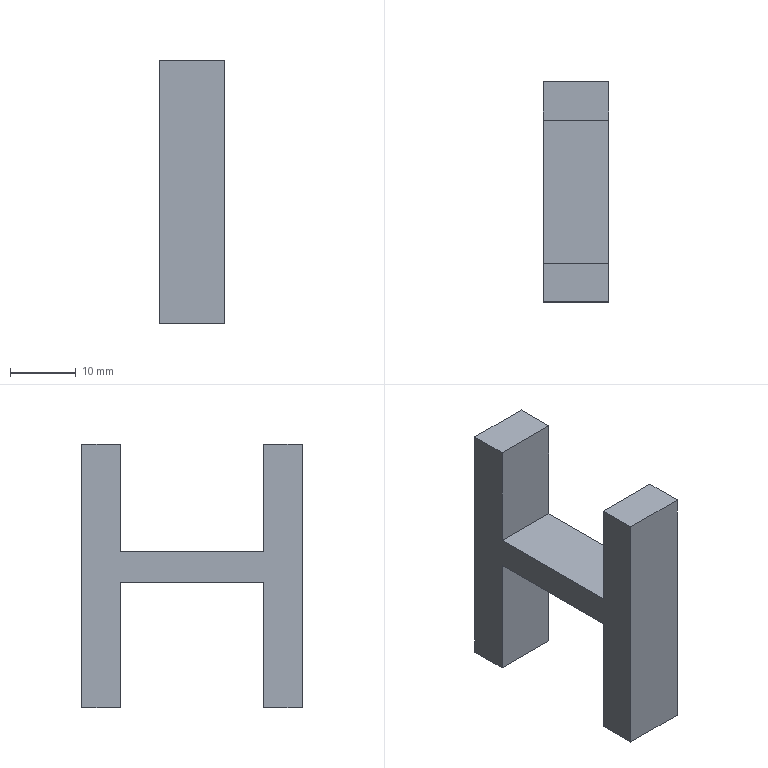Part | NX | features solid 2 | 1 solid | 14 faces | box 10 x 33.468 x 40 mm | volume 5698 mm3 | plane 14
STEP:
#1=CARTESIAN_POINT('',(2250.,-874.141,-590.));
#2=VERTEX_POINT('',#1);
#3=CARTESIAN_POINT('',(2250.,-880.,-590.));
#4=VERTEX_POINT('',#3);
#5=CARTESIAN_POINT('',(2250.,-874.141,-590.));
#6=CARTESIAN_POINT('',(2250.,-876.094,-590.));
#7=CARTESIAN_POINT('',(2250.,-878.047,-590.));
#8=CARTESIAN_POINT('',(2250.,-880.,-590.));
#9=B_SPLINE_CURVE_WITH_KNOTS('',3,(#5,#6,#7,#8),.UNSPECIFIED.,.F.,.F.,(4,4),(0.,0.02692),.PIECEWISE_BEZIER_KNOTS.);
#10=EDGE_CURVE('',#2,#4,#9,.T.);
#11=ORIENTED_EDGE('',*,*,#10,.F.);
#12=CARTESIAN_POINT('',(2260.,-874.141,-590.));
#13=VERTEX_POINT('',#12);
#14=CARTESIAN_POINT('',(2260.,-874.141,-590.));
#15=DIRECTION('',(-1.,0.,0.));
#16=VECTOR('',#15,1000.);
#17=LINE('',#14,#16);
#18=EDGE_CURVE('',#13,#2,#17,.T.);
#19=ORIENTED_EDGE('',*,*,#18,.F.);
#20=CARTESIAN_POINT('',(2260.,-880.,-590.));
#21=VERTEX_POINT('',#20);
#22=CARTESIAN_POINT('',(2260.,-874.141,-590.));
#23=CARTESIAN_POINT('',(2260.,-876.094,-590.));
#24=CARTESIAN_POINT('',(2260.,-878.047,-590.));
#25=CARTESIAN_POINT('',(2260.,-880.,-590.));
#26=B_SPLINE_CURVE_WITH_KNOTS('',3,(#22,#23,#24,#25),.UNSPECIFIED.,.F.,.F.,(4,4),(0.,0.02692),.PIECEWISE_BEZIER_KNOTS.);
#27=EDGE_CURVE('',#13,#21,#26,.T.);
#28=ORIENTED_EDGE('',*,*,#27,.T.);
#29=CARTESIAN_POINT('',(2260.,-880.,-590.));
#30=DIRECTION('',(-1.,0.,0.));
#31=VECTOR('',#30,1000.);
#32=LINE('',#29,#31);
#33=EDGE_CURVE('',#21,#4,#32,.T.);
#34=ORIENTED_EDGE('',*,*,#33,.T.);
#35=EDGE_LOOP('',(#11,#19,#28,#34));
#36=FACE_BOUND('',#35,.T.);
#37=CARTESIAN_POINT('',(2260.,-874.141,-590.));
#38=DIRECTION('',(0.,0.,-1.));
#39=DIRECTION('',(-1.,0.,0.));
#40=AXIS2_PLACEMENT_3D('',#37,#38,#39);
#41=PLANE('',#40);
#42=ADVANCED_FACE('',(#36),#41,.T.);
#43=CARTESIAN_POINT('',(2250.,-880.,-550.));
#44=VERTEX_POINT('',#43);
#45=CARTESIAN_POINT('',(2250.,-880.,-590.));
#46=CARTESIAN_POINT('',(2250.,-880.,-576.667));
#47=CARTESIAN_POINT('',(2250.,-880.,-563.333));
#48=CARTESIAN_POINT('',(2250.,-880.,-550.));
#49=B_SPLINE_CURVE_WITH_KNOTS('',3,(#45,#46,#47,#48),.UNSPECIFIED.,.F.,.F.,(4,4),(0.02692,0.2107),.PIECEWISE_BEZIER_KNOTS.);
#50=EDGE_CURVE('',#4,#44,#49,.T.);
#51=ORIENTED_EDGE('',*,*,#50,.F.);
#52=ORIENTED_EDGE('',*,*,#33,.F.);
#53=CARTESIAN_POINT('',(2260.,-880.,-550.));
#54=VERTEX_POINT('',#53);
#55=CARTESIAN_POINT('',(2260.,-880.,-590.));
#56=CARTESIAN_POINT('',(2260.,-880.,-576.667));
#57=CARTESIAN_POINT('',(2260.,-880.,-563.333));
#58=CARTESIAN_POINT('',(2260.,-880.,-550.));
#59=B_SPLINE_CURVE_WITH_KNOTS('',3,(#55,#56,#57,#58),.UNSPECIFIED.,.F.,.F.,(4,4),(0.02692,0.2107),.PIECEWISE_BEZIER_KNOTS.);
#60=EDGE_CURVE('',#21,#54,#59,.T.);
#61=ORIENTED_EDGE('',*,*,#60,.T.);
#62=CARTESIAN_POINT('',(2260.,-880.,-550.));
#63=DIRECTION('',(-1.,0.,0.));
#64=VECTOR('',#63,1000.);
#65=LINE('',#62,#64);
#66=EDGE_CURVE('',#54,#44,#65,.T.);
#67=ORIENTED_EDGE('',*,*,#66,.T.);
#68=EDGE_LOOP('',(#51,#52,#61,#67));
#69=FACE_BOUND('',#68,.T.);
#70=CARTESIAN_POINT('',(2260.,-880.,-590.));
#71=DIRECTION('',(0.,-1.,0.));
#72=DIRECTION('',(1.,0.,0.));
#73=AXIS2_PLACEMENT_3D('',#70,#71,#72);
#74=PLANE('',#73);
#75=ADVANCED_FACE('',(#69),#74,.T.);
#76=CARTESIAN_POINT('',(2250.,-874.141,-550.));
#77=VERTEX_POINT('',#76);
#78=CARTESIAN_POINT('',(2250.,-880.,-550.));
#79=CARTESIAN_POINT('',(2250.,-878.047,-550.));
#80=CARTESIAN_POINT('',(2250.,-876.094,-550.));
#81=CARTESIAN_POINT('',(2250.,-874.141,-550.));
#82=B_SPLINE_CURVE_WITH_KNOTS('',3,(#78,#79,#80,#81),.UNSPECIFIED.,.F.,.F.,(4,4),(0.2107,0.2376),.PIECEWISE_BEZIER_KNOTS.);
#83=EDGE_CURVE('',#44,#77,#82,.T.);
#84=ORIENTED_EDGE('',*,*,#83,.F.);
#85=ORIENTED_EDGE('',*,*,#66,.F.);
#86=CARTESIAN_POINT('',(2260.,-874.141,-550.));
#87=VERTEX_POINT('',#86);
#88=CARTESIAN_POINT('',(2260.,-880.,-550.));
#89=CARTESIAN_POINT('',(2260.,-878.047,-550.));
#90=CARTESIAN_POINT('',(2260.,-876.094,-550.));
#91=CARTESIAN_POINT('',(2260.,-874.141,-550.));
#92=B_SPLINE_CURVE_WITH_KNOTS('',3,(#88,#89,#90,#91),.UNSPECIFIED.,.F.,.F.,(4,4),(0.2107,0.2376),.PIECEWISE_BEZIER_KNOTS.);
#93=EDGE_CURVE('',#54,#87,#92,.T.);
#94=ORIENTED_EDGE('',*,*,#93,.T.);
#95=CARTESIAN_POINT('',(2260.,-874.141,-550.));
#96=DIRECTION('',(-1.,0.,0.));
#97=VECTOR('',#96,1000.);
#98=LINE('',#95,#97);
#99=EDGE_CURVE('',#87,#77,#98,.T.);
#100=ORIENTED_EDGE('',*,*,#99,.T.);
#101=EDGE_LOOP('',(#84,#85,#94,#100));
#102=FACE_BOUND('',#101,.T.);
#103=CARTESIAN_POINT('',(2260.,-880.,-550.));
#104=DIRECTION('',(0.,0.,1.));
#105=DIRECTION('',(1.,0.,0.));
#106=AXIS2_PLACEMENT_3D('',#103,#104,#105);
#107=PLANE('',#106);
#108=ADVANCED_FACE('',(#102),#107,.T.);
#109=CARTESIAN_POINT('',(2250.,-874.141,-566.321));
#110=VERTEX_POINT('',#109);
#111=CARTESIAN_POINT('',(2250.,-874.141,-550.));
#112=CARTESIAN_POINT('',(2250.,-874.141,-555.44));
#113=CARTESIAN_POINT('',(2250.,-874.141,-560.881));
#114=CARTESIAN_POINT('',(2250.,-874.141,-566.321));
#115=B_SPLINE_CURVE_WITH_KNOTS('',3,(#111,#112,#113,#114),.UNSPECIFIED.,.F.,.F.,(4,4),(0.2376,0.3126),.PIECEWISE_BEZIER_KNOTS.);
#116=EDGE_CURVE('',#77,#110,#115,.T.);
#117=ORIENTED_EDGE('',*,*,#116,.F.);
#118=ORIENTED_EDGE('',*,*,#99,.F.);
#119=CARTESIAN_POINT('',(2260.,-874.141,-566.321));
#120=VERTEX_POINT('',#119);
#121=CARTESIAN_POINT('',(2260.,-874.141,-550.));
#122=CARTESIAN_POINT('',(2260.,-874.141,-555.44));
#123=CARTESIAN_POINT('',(2260.,-874.141,-560.881));
#124=CARTESIAN_POINT('',(2260.,-874.141,-566.321));
#125=B_SPLINE_CURVE_WITH_KNOTS('',3,(#121,#122,#123,#124),.UNSPECIFIED.,.F.,.F.,(4,4),(0.2376,0.3126),.PIECEWISE_BEZIER_KNOTS.);
#126=EDGE_CURVE('',#87,#120,#125,.T.);
#127=ORIENTED_EDGE('',*,*,#126,.T.);
#128=CARTESIAN_POINT('',(2260.,-874.141,-566.321));
#129=DIRECTION('',(-1.,0.,0.));
#130=VECTOR('',#129,1000.);
#131=LINE('',#128,#130);
#132=EDGE_CURVE('',#120,#110,#131,.T.);
#133=ORIENTED_EDGE('',*,*,#132,.T.);
#134=EDGE_LOOP('',(#117,#118,#127,#133));
#135=FACE_BOUND('',#134,.T.);
#136=CARTESIAN_POINT('',(2260.,-874.141,-550.));
#137=DIRECTION('',(0.,1.,0.));
#138=DIRECTION('',(-1.,0.,0.));
#139=AXIS2_PLACEMENT_3D('',#136,#137,#138);
#140=PLANE('',#139);
#141=ADVANCED_FACE('',(#135),#140,.T.);
#142=CARTESIAN_POINT('',(2250.,-852.39,-566.321));
#143=VERTEX_POINT('',#142);
#144=CARTESIAN_POINT('',(2250.,-874.141,-566.321));
#145=CARTESIAN_POINT('',(2250.,-866.891,-566.321));
#146=CARTESIAN_POINT('',(2250.,-859.641,-566.321));
#147=CARTESIAN_POINT('',(2250.,-852.39,-566.321));
#148=B_SPLINE_CURVE_WITH_KNOTS('',3,(#144,#145,#146,#147),.UNSPECIFIED.,.F.,.F.,(4,4),(0.3126,0.4126),.PIECEWISE_BEZIER_KNOTS.);
#149=EDGE_CURVE('',#110,#143,#148,.T.);
#150=ORIENTED_EDGE('',*,*,#149,.F.);
#151=ORIENTED_EDGE('',*,*,#132,.F.);
#152=CARTESIAN_POINT('',(2260.,-852.39,-566.321));
#153=VERTEX_POINT('',#152);
#154=CARTESIAN_POINT('',(2260.,-874.141,-566.321));
#155=CARTESIAN_POINT('',(2260.,-866.891,-566.321));
#156=CARTESIAN_POINT('',(2260.,-859.641,-566.321));
#157=CARTESIAN_POINT('',(2260.,-852.39,-566.321));
#158=B_SPLINE_CURVE_WITH_KNOTS('',3,(#154,#155,#156,#157),.UNSPECIFIED.,.F.,.F.,(4,4),(0.3126,0.4126),.PIECEWISE_BEZIER_KNOTS.);
#159=EDGE_CURVE('',#120,#153,#158,.T.);
#160=ORIENTED_EDGE('',*,*,#159,.T.);
#161=CARTESIAN_POINT('',(2260.,-852.39,-566.321));
#162=DIRECTION('',(-1.,0.,0.));
#163=VECTOR('',#162,1000.);
#164=LINE('',#161,#163);
#165=EDGE_CURVE('',#153,#143,#164,.T.);
#166=ORIENTED_EDGE('',*,*,#165,.T.);
#167=EDGE_LOOP('',(#150,#151,#160,#166));
#168=FACE_BOUND('',#167,.T.);
#169=CARTESIAN_POINT('',(2260.,-874.141,-566.321));
#170=DIRECTION('',(0.,0.,1.));
#171=DIRECTION('',(1.,0.,0.));
#172=AXIS2_PLACEMENT_3D('',#169,#170,#171);
#173=PLANE('',#172);
#174=ADVANCED_FACE('',(#168),#173,.T.);
#175=CARTESIAN_POINT('',(2250.,-852.39,-550.));
#176=VERTEX_POINT('',#175);
#177=CARTESIAN_POINT('',(2250.,-852.39,-566.321));
#178=CARTESIAN_POINT('',(2250.,-852.39,-560.881));
#179=CARTESIAN_POINT('',(2250.,-852.39,-555.44));
#180=CARTESIAN_POINT('',(2250.,-852.39,-550.));
#181=B_SPLINE_CURVE_WITH_KNOTS('',3,(#177,#178,#179,#180),.UNSPECIFIED.,.F.,.F.,(4,4),(0.4126,0.4876),.PIECEWISE_BEZIER_KNOTS.);
#182=EDGE_CURVE('',#143,#176,#181,.T.);
#183=ORIENTED_EDGE('',*,*,#182,.F.);
#184=ORIENTED_EDGE('',*,*,#165,.F.);
#185=CARTESIAN_POINT('',(2260.,-852.39,-550.));
#186=VERTEX_POINT('',#185);
#187=CARTESIAN_POINT('',(2260.,-852.39,-566.321));
#188=CARTESIAN_POINT('',(2260.,-852.39,-560.881));
#189=CARTESIAN_POINT('',(2260.,-852.39,-555.44));
#190=CARTESIAN_POINT('',(2260.,-852.39,-550.));
#191=B_SPLINE_CURVE_WITH_KNOTS('',3,(#187,#188,#189,#190),.UNSPECIFIED.,.F.,.F.,(4,4),(0.4126,0.4876),.PIECEWISE_BEZIER_KNOTS.);
#192=EDGE_CURVE('',#153,#186,#191,.T.);
#193=ORIENTED_EDGE('',*,*,#192,.T.);
#194=CARTESIAN_POINT('',(2260.,-852.39,-550.));
#195=DIRECTION('',(-1.,0.,0.));
#196=VECTOR('',#195,1000.);
#197=LINE('',#194,#196);
#198=EDGE_CURVE('',#186,#176,#197,.T.);
#199=ORIENTED_EDGE('',*,*,#198,.T.);
#200=EDGE_LOOP('',(#183,#184,#193,#199));
#201=FACE_BOUND('',#200,.T.);
#202=CARTESIAN_POINT('',(2260.,-852.39,-566.321));
#203=DIRECTION('',(0.,-1.,0.));
#204=DIRECTION('',(1.,0.,0.));
#205=AXIS2_PLACEMENT_3D('',#202,#203,#204);
#206=PLANE('',#205);
#207=ADVANCED_FACE('',(#201),#206,.T.);
#208=CARTESIAN_POINT('',(2250.,-846.532,-550.));
#209=VERTEX_POINT('',#208);
#210=CARTESIAN_POINT('',(2250.,-852.39,-550.));
#211=CARTESIAN_POINT('',(2250.,-850.437,-550.));
#212=CARTESIAN_POINT('',(2250.,-848.484,-550.));
#213=CARTESIAN_POINT('',(2250.,-846.532,-550.));
#214=B_SPLINE_CURVE_WITH_KNOTS('',3,(#210,#211,#212,#213),.UNSPECIFIED.,.F.,.F.,(4,4),(0.4876,0.5145),.PIECEWISE_BEZIER_KNOTS.);
#215=EDGE_CURVE('',#176,#209,#214,.T.);
#216=ORIENTED_EDGE('',*,*,#215,.F.);
#217=ORIENTED_EDGE('',*,*,#198,.F.);
#218=CARTESIAN_POINT('',(2260.,-846.532,-550.));
#219=VERTEX_POINT('',#218);
#220=CARTESIAN_POINT('',(2260.,-852.39,-550.));
#221=CARTESIAN_POINT('',(2260.,-850.437,-550.));
#222=CARTESIAN_POINT('',(2260.,-848.484,-550.));
#223=CARTESIAN_POINT('',(2260.,-846.532,-550.));
#224=B_SPLINE_CURVE_WITH_KNOTS('',3,(#220,#221,#222,#223),.UNSPECIFIED.,.F.,.F.,(4,4),(0.4876,0.5145),.PIECEWISE_BEZIER_KNOTS.);
#225=EDGE_CURVE('',#186,#219,#224,.T.);
#226=ORIENTED_EDGE('',*,*,#225,.T.);
#227=CARTESIAN_POINT('',(2260.,-846.532,-550.));
#228=DIRECTION('',(-1.,0.,0.));
#229=VECTOR('',#228,1000.);
#230=LINE('',#227,#229);
#231=EDGE_CURVE('',#219,#209,#230,.T.);
#232=ORIENTED_EDGE('',*,*,#231,.T.);
#233=EDGE_LOOP('',(#216,#217,#226,#232));
#234=FACE_BOUND('',#233,.T.);
#235=CARTESIAN_POINT('',(2260.,-852.39,-550.));
#236=DIRECTION('',(0.,0.,1.));
#237=DIRECTION('',(1.,0.,0.));
#238=AXIS2_PLACEMENT_3D('',#235,#236,#237);
#239=PLANE('',#238);
#240=ADVANCED_FACE('',(#234),#239,.T.);
#241=CARTESIAN_POINT('',(2250.,-846.532,-590.));
#242=VERTEX_POINT('',#241);
#243=CARTESIAN_POINT('',(2250.,-846.532,-550.));
#244=CARTESIAN_POINT('',(2250.,-846.532,-563.333));
#245=CARTESIAN_POINT('',(2250.,-846.532,-576.667));
#246=CARTESIAN_POINT('',(2250.,-846.532,-590.));
#247=B_SPLINE_CURVE_WITH_KNOTS('',3,(#243,#244,#245,#246),.UNSPECIFIED.,.F.,.F.,(4,4),(0.5145,0.6983),.PIECEWISE_BEZIER_KNOTS.);
#248=EDGE_CURVE('',#209,#242,#247,.T.);
#249=ORIENTED_EDGE('',*,*,#248,.F.);
#250=ORIENTED_EDGE('',*,*,#231,.F.);
#251=CARTESIAN_POINT('',(2260.,-846.532,-590.));
#252=VERTEX_POINT('',#251);
#253=CARTESIAN_POINT('',(2260.,-846.532,-550.));
#254=CARTESIAN_POINT('',(2260.,-846.532,-563.333));
#255=CARTESIAN_POINT('',(2260.,-846.532,-576.667));
#256=CARTESIAN_POINT('',(2260.,-846.532,-590.));
#257=B_SPLINE_CURVE_WITH_KNOTS('',3,(#253,#254,#255,#256),.UNSPECIFIED.,.F.,.F.,(4,4),(0.5145,0.6983),.PIECEWISE_BEZIER_KNOTS.);
#258=EDGE_CURVE('',#219,#252,#257,.T.);
#259=ORIENTED_EDGE('',*,*,#258,.T.);
#260=CARTESIAN_POINT('',(2260.,-846.532,-590.));
#261=DIRECTION('',(-1.,0.,0.));
#262=VECTOR('',#261,1000.);
#263=LINE('',#260,#262);
#264=EDGE_CURVE('',#252,#242,#263,.T.);
#265=ORIENTED_EDGE('',*,*,#264,.T.);
#266=EDGE_LOOP('',(#249,#250,#259,#265));
#267=FACE_BOUND('',#266,.T.);
#268=CARTESIAN_POINT('',(2260.,-846.532,-550.));
#269=DIRECTION('',(0.,1.,0.));
#270=DIRECTION('',(-1.,0.,0.));
#271=AXIS2_PLACEMENT_3D('',#268,#269,#270);
#272=PLANE('',#271);
#273=ADVANCED_FACE('',(#267),#272,.T.);
#274=CARTESIAN_POINT('',(2250.,-852.39,-590.));
#275=VERTEX_POINT('',#274);
#276=CARTESIAN_POINT('',(2250.,-846.532,-590.));
#277=CARTESIAN_POINT('',(2250.,-848.484,-590.));
#278=CARTESIAN_POINT('',(2250.,-850.437,-590.));
#279=CARTESIAN_POINT('',(2250.,-852.39,-590.));
#280=B_SPLINE_CURVE_WITH_KNOTS('',3,(#276,#277,#278,#279),.UNSPECIFIED.,.F.,.F.,(4,4),(0.6983,0.7252),.PIECEWISE_BEZIER_KNOTS.);
#281=EDGE_CURVE('',#242,#275,#280,.T.);
#282=ORIENTED_EDGE('',*,*,#281,.F.);
#283=ORIENTED_EDGE('',*,*,#264,.F.);
#284=CARTESIAN_POINT('',(2260.,-852.39,-590.));
#285=VERTEX_POINT('',#284);
#286=CARTESIAN_POINT('',(2260.,-846.532,-590.));
#287=CARTESIAN_POINT('',(2260.,-848.484,-590.));
#288=CARTESIAN_POINT('',(2260.,-850.437,-590.));
#289=CARTESIAN_POINT('',(2260.,-852.39,-590.));
#290=B_SPLINE_CURVE_WITH_KNOTS('',3,(#286,#287,#288,#289),.UNSPECIFIED.,.F.,.F.,(4,4),(0.6983,0.7252),.PIECEWISE_BEZIER_KNOTS.);
#291=EDGE_CURVE('',#252,#285,#290,.T.);
#292=ORIENTED_EDGE('',*,*,#291,.T.);
#293=CARTESIAN_POINT('',(2260.,-852.39,-590.));
#294=DIRECTION('',(-1.,0.,0.));
#295=VECTOR('',#294,1000.);
#296=LINE('',#293,#295);
#297=EDGE_CURVE('',#285,#275,#296,.T.);
#298=ORIENTED_EDGE('',*,*,#297,.T.);
#299=EDGE_LOOP('',(#282,#283,#292,#298));
#300=FACE_BOUND('',#299,.T.);
#301=CARTESIAN_POINT('',(2260.,-846.532,-590.));
#302=DIRECTION('',(0.,0.,-1.));
#303=DIRECTION('',(-1.,0.,0.));
#304=AXIS2_PLACEMENT_3D('',#301,#302,#303);
#305=PLANE('',#304);
#306=ADVANCED_FACE('',(#300),#305,.T.);
#307=CARTESIAN_POINT('',(2250.,-852.39,-570.971));
#308=VERTEX_POINT('',#307);
#309=CARTESIAN_POINT('',(2250.,-852.39,-590.));
#310=CARTESIAN_POINT('',(2250.,-852.39,-583.657));
#311=CARTESIAN_POINT('',(2250.,-852.39,-577.314));
#312=CARTESIAN_POINT('',(2250.,-852.39,-570.971));
#313=B_SPLINE_CURVE_WITH_KNOTS('',3,(#309,#310,#311,#312),.UNSPECIFIED.,.F.,.F.,(4,4),(0.7252,0.8126),.PIECEWISE_BEZIER_KNOTS.);
#314=EDGE_CURVE('',#275,#308,#313,.T.);
#315=ORIENTED_EDGE('',*,*,#314,.F.);
#316=ORIENTED_EDGE('',*,*,#297,.F.);
#317=CARTESIAN_POINT('',(2260.,-852.39,-570.971));
#318=VERTEX_POINT('',#317);
#319=CARTESIAN_POINT('',(2260.,-852.39,-590.));
#320=CARTESIAN_POINT('',(2260.,-852.39,-583.657));
#321=CARTESIAN_POINT('',(2260.,-852.39,-577.314));
#322=CARTESIAN_POINT('',(2260.,-852.39,-570.971));
#323=B_SPLINE_CURVE_WITH_KNOTS('',3,(#319,#320,#321,#322),.UNSPECIFIED.,.F.,.F.,(4,4),(0.7252,0.8126),.PIECEWISE_BEZIER_KNOTS.);
#324=EDGE_CURVE('',#285,#318,#323,.T.);
#325=ORIENTED_EDGE('',*,*,#324,.T.);
#326=CARTESIAN_POINT('',(2260.,-852.39,-570.971));
#327=DIRECTION('',(-1.,0.,0.));
#328=VECTOR('',#327,1000.);
#329=LINE('',#326,#328);
#330=EDGE_CURVE('',#318,#308,#329,.T.);
#331=ORIENTED_EDGE('',*,*,#330,.T.);
#332=EDGE_LOOP('',(#315,#316,#325,#331));
#333=FACE_BOUND('',#332,.T.);
#334=CARTESIAN_POINT('',(2260.,-852.39,-590.));
#335=DIRECTION('',(0.,-1.,0.));
#336=DIRECTION('',(1.,0.,0.));
#337=AXIS2_PLACEMENT_3D('',#334,#335,#336);
#338=PLANE('',#337);
#339=ADVANCED_FACE('',(#333),#338,.T.);
#340=CARTESIAN_POINT('',(2250.,-874.141,-570.971));
#341=VERTEX_POINT('',#340);
#342=CARTESIAN_POINT('',(2250.,-852.39,-570.971));
#343=CARTESIAN_POINT('',(2250.,-859.641,-570.971));
#344=CARTESIAN_POINT('',(2250.,-866.891,-570.971));
#345=CARTESIAN_POINT('',(2250.,-874.141,-570.971));
#346=B_SPLINE_CURVE_WITH_KNOTS('',3,(#342,#343,#344,#345),.UNSPECIFIED.,.F.,.F.,(4,4),(0.8126,0.9126),.PIECEWISE_BEZIER_KNOTS.);
#347=EDGE_CURVE('',#308,#341,#346,.T.);
#348=ORIENTED_EDGE('',*,*,#347,.F.);
#349=ORIENTED_EDGE('',*,*,#330,.F.);
#350=CARTESIAN_POINT('',(2260.,-874.141,-570.971));
#351=VERTEX_POINT('',#350);
#352=CARTESIAN_POINT('',(2260.,-852.39,-570.971));
#353=CARTESIAN_POINT('',(2260.,-859.641,-570.971));
#354=CARTESIAN_POINT('',(2260.,-866.891,-570.971));
#355=CARTESIAN_POINT('',(2260.,-874.141,-570.971));
#356=B_SPLINE_CURVE_WITH_KNOTS('',3,(#352,#353,#354,#355),.UNSPECIFIED.,.F.,.F.,(4,4),(0.8126,0.9126),.PIECEWISE_BEZIER_KNOTS.);
#357=EDGE_CURVE('',#318,#351,#356,.T.);
#358=ORIENTED_EDGE('',*,*,#357,.T.);
#359=CARTESIAN_POINT('',(2260.,-874.141,-570.971));
#360=DIRECTION('',(-1.,0.,0.));
#361=VECTOR('',#360,1000.);
#362=LINE('',#359,#361);
#363=EDGE_CURVE('',#351,#341,#362,.T.);
#364=ORIENTED_EDGE('',*,*,#363,.T.);
#365=EDGE_LOOP('',(#348,#349,#358,#364));
#366=FACE_BOUND('',#365,.T.);
#367=CARTESIAN_POINT('',(2260.,-852.39,-570.971));
#368=DIRECTION('',(0.,0.,-1.));
#369=DIRECTION('',(-1.,0.,0.));
#370=AXIS2_PLACEMENT_3D('',#367,#368,#369);
#371=PLANE('',#370);
#372=ADVANCED_FACE('',(#366),#371,.T.);
#373=CARTESIAN_POINT('',(2250.,-874.141,-570.971));
#374=CARTESIAN_POINT('',(2250.,-874.141,-577.314));
#375=CARTESIAN_POINT('',(2250.,-874.141,-583.657));
#376=CARTESIAN_POINT('',(2250.,-874.141,-590.));
#377=B_SPLINE_CURVE_WITH_KNOTS('',3,(#373,#374,#375,#376),.UNSPECIFIED.,.F.,.F.,(4,4),(0.9126,1.),.PIECEWISE_BEZIER_KNOTS.);
#378=EDGE_CURVE('',#341,#2,#377,.T.);
#379=ORIENTED_EDGE('',*,*,#378,.F.);
#380=ORIENTED_EDGE('',*,*,#363,.F.);
#381=CARTESIAN_POINT('',(2260.,-874.141,-570.971));
#382=CARTESIAN_POINT('',(2260.,-874.141,-577.314));
#383=CARTESIAN_POINT('',(2260.,-874.141,-583.657));
#384=CARTESIAN_POINT('',(2260.,-874.141,-590.));
#385=B_SPLINE_CURVE_WITH_KNOTS('',3,(#381,#382,#383,#384),.UNSPECIFIED.,.F.,.F.,(4,4),(0.9126,1.),.PIECEWISE_BEZIER_KNOTS.);
#386=EDGE_CURVE('',#351,#13,#385,.T.);
#387=ORIENTED_EDGE('',*,*,#386,.T.);
#388=ORIENTED_EDGE('',*,*,#18,.T.);
#389=EDGE_LOOP('',(#379,#380,#387,#388));
#390=FACE_BOUND('',#389,.T.);
#391=CARTESIAN_POINT('',(2260.,-874.141,-570.971));
#392=DIRECTION('',(0.,1.,0.));
#393=DIRECTION('',(-1.,0.,0.));
#394=AXIS2_PLACEMENT_3D('',#391,#392,#393);
#395=PLANE('',#394);
#396=ADVANCED_FACE('',(#390),#395,.T.);
#397=ORIENTED_EDGE('',*,*,#27,.F.);
#398=ORIENTED_EDGE('',*,*,#386,.F.);
#399=ORIENTED_EDGE('',*,*,#357,.F.);
#400=ORIENTED_EDGE('',*,*,#324,.F.);
#401=ORIENTED_EDGE('',*,*,#291,.F.);
#402=ORIENTED_EDGE('',*,*,#258,.F.);
#403=ORIENTED_EDGE('',*,*,#225,.F.);
#404=ORIENTED_EDGE('',*,*,#192,.F.);
#405=ORIENTED_EDGE('',*,*,#159,.F.);
#406=ORIENTED_EDGE('',*,*,#126,.F.);
#407=ORIENTED_EDGE('',*,*,#93,.F.);
#408=ORIENTED_EDGE('',*,*,#60,.F.);
#409=EDGE_LOOP('',(#397,#398,#399,#400,#401,#402,#403,#404,#405,#406,#407,#408));
#410=FACE_BOUND('',#409,.T.);
#411=CARTESIAN_POINT('',(2260.,-877.071,-590.));
#412=DIRECTION('',(1.,0.,0.));
#413=DIRECTION('',(0.,1.,0.));
#414=AXIS2_PLACEMENT_3D('',#411,#412,#413);
#415=PLANE('',#414);
#416=ADVANCED_FACE('',(#410),#415,.T.);
#417=ORIENTED_EDGE('',*,*,#10,.T.);
#418=ORIENTED_EDGE('',*,*,#50,.T.);
#419=ORIENTED_EDGE('',*,*,#83,.T.);
#420=ORIENTED_EDGE('',*,*,#116,.T.);
#421=ORIENTED_EDGE('',*,*,#149,.T.);
#422=ORIENTED_EDGE('',*,*,#182,.T.);
#423=ORIENTED_EDGE('',*,*,#215,.T.);
#424=ORIENTED_EDGE('',*,*,#248,.T.);
#425=ORIENTED_EDGE('',*,*,#281,.T.);
#426=ORIENTED_EDGE('',*,*,#314,.T.);
#427=ORIENTED_EDGE('',*,*,#347,.T.);
#428=ORIENTED_EDGE('',*,*,#378,.T.);
#429=EDGE_LOOP('',(#417,#418,#419,#420,#421,#422,#423,#424,#425,#426,#427,#428));
#430=FACE_BOUND('',#429,.T.);
#431=CARTESIAN_POINT('',(2250.,-877.071,-590.));
#432=DIRECTION('',(1.,0.,0.));
#433=DIRECTION('',(0.,1.,0.));
#434=AXIS2_PLACEMENT_3D('',#431,#432,#433);
#435=PLANE('',#434);
#436=ADVANCED_FACE('',(#430),#435,.F.);
#437=CLOSED_SHELL('',(#42,#75,#108,#141,#174,#207,#240,#273,#306,#339,#372,#396,#416,#436));
#438=MANIFOLD_SOLID_BREP('',#437);
#439=(LENGTH_UNIT()NAMED_UNIT(*)SI_UNIT(.MILLI.,.METRE.));
#440=UNCERTAINTY_MEASURE_WITH_UNIT(LENGTH_MEASURE(0.00001),#439,'','');
#441=(NAMED_UNIT(*)PLANE_ANGLE_UNIT()SI_UNIT($,.RADIAN.));
#442=(NAMED_UNIT(*)SI_UNIT($,.STERADIAN.)SOLID_ANGLE_UNIT());
#443=(GEOMETRIC_REPRESENTATION_CONTEXT(3)GLOBAL_UNCERTAINTY_ASSIGNED_CONTEXT((#440))GLOBAL_UNIT_ASSIGNED_CONTEXT((#439,#441,#442))REPRESENTATION_CONTEXT('',''));
#444=ADVANCED_BREP_SHAPE_REPRESENTATION('',(#438),#443);